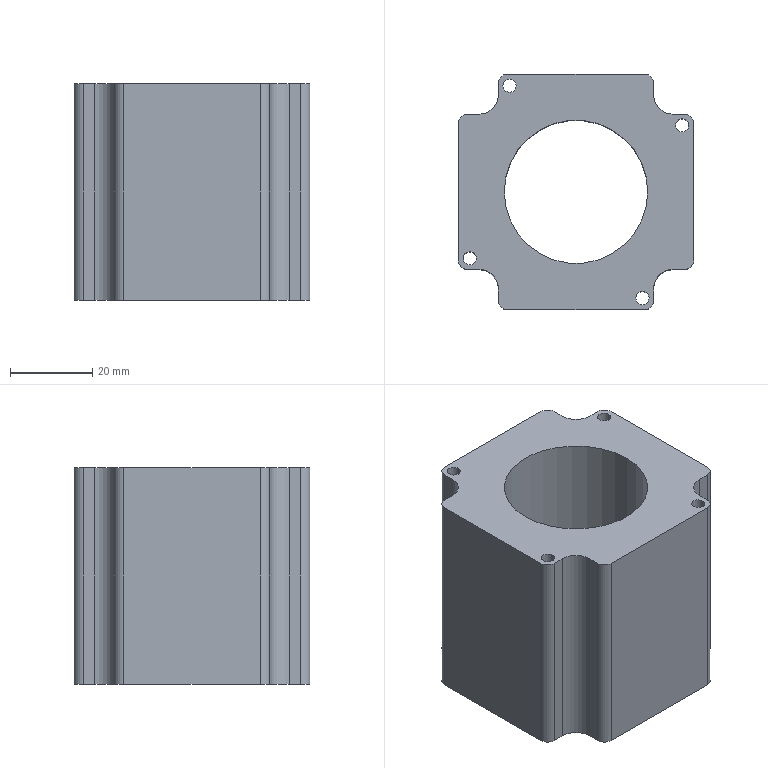Part | NX | features BREP 1 | 1 solid | 36 faces | box 57.15 x 57.15 x 52.6 mm | volume 100652 mm3 | cylinder 22 | plane 14 | commonest cylinder face diameters 3.2 x8 4.6 x8 9.5 x4 34.78 x2
STEP:
#1=CARTESIAN_POINT('',(17.39,0.,52.6));
#2=VERTEX_POINT('',#1);
#3=CARTESIAN_POINT('',(-17.39,0.,52.6));
#4=VERTEX_POINT('',#3);
#5=CARTESIAN_POINT('',(0.,0.,52.6));
#6=DIRECTION('',(0.,0.,-1.));
#7=DIRECTION('',(-1.,0.,0.));
#8=AXIS2_PLACEMENT_3D('',#5,#6,#7);
#9=CIRCLE('',#8,17.39);
#10=EDGE_CURVE('',#2,#4,#9,.T.);
#11=ORIENTED_EDGE('',*,*,#10,.F.);
#12=CARTESIAN_POINT('',(17.39,0.,0.));
#13=VERTEX_POINT('',#12);
#14=CARTESIAN_POINT('',(17.39,0.,52.6));
#15=DIRECTION('',(0.,0.,-1.));
#16=VECTOR('',#15,1000.);
#17=LINE('',#14,#16);
#18=EDGE_CURVE('',#13,#2,#17,.F.);
#19=ORIENTED_EDGE('',*,*,#18,.F.);
#20=CARTESIAN_POINT('',(-17.39,0.,0.));
#21=VERTEX_POINT('',#20);
#22=CARTESIAN_POINT('',(0.,0.,0.));
#23=DIRECTION('',(0.,0.,1.));
#24=DIRECTION('',(-1.,0.,0.));
#25=AXIS2_PLACEMENT_3D('',#22,#23,#24);
#26=CIRCLE('',#25,17.39);
#27=EDGE_CURVE('',#21,#13,#26,.T.);
#28=ORIENTED_EDGE('',*,*,#27,.F.);
#29=CARTESIAN_POINT('',(-17.39,0.,52.6));
#30=DIRECTION('',(0.,0.,-1.));
#31=VECTOR('',#30,1000.);
#32=LINE('',#29,#31);
#33=EDGE_CURVE('',#21,#4,#32,.F.);
#34=ORIENTED_EDGE('',*,*,#33,.T.);
#35=EDGE_LOOP('',(#11,#19,#28,#34));
#36=FACE_BOUND('',#35,.T.);
#37=CARTESIAN_POINT('',(0.,0.,52.6));
#38=DIRECTION('',(0.,0.,-1.));
#39=DIRECTION('',(1.,0.,0.));
#40=AXIS2_PLACEMENT_3D('',#37,#38,#39);
#41=CYLINDRICAL_SURFACE('',#40,17.39);
#42=ADVANCED_FACE('',(#36),#41,.F.);
#43=CARTESIAN_POINT('',(-14.51,25.75,0.));
#44=VERTEX_POINT('',#43);
#45=CARTESIAN_POINT('',(-17.71,25.75,0.));
#46=VERTEX_POINT('',#45);
#47=CARTESIAN_POINT('',(-16.11,25.75,0.));
#48=DIRECTION('',(0.,0.,-1.));
#49=DIRECTION('',(1.,0.,0.));
#50=AXIS2_PLACEMENT_3D('',#47,#48,#49);
#51=CIRCLE('',#50,1.6);
#52=EDGE_CURVE('',#44,#46,#51,.T.);
#53=ORIENTED_EDGE('',*,*,#52,.T.);
#54=CARTESIAN_POINT('',(-17.71,25.75,52.6));
#55=VERTEX_POINT('',#54);
#56=CARTESIAN_POINT('',(-17.71,25.75,0.));
#57=DIRECTION('',(0.,0.,1.));
#58=VECTOR('',#57,1000.);
#59=LINE('',#56,#58);
#60=EDGE_CURVE('',#46,#55,#59,.T.);
#61=ORIENTED_EDGE('',*,*,#60,.T.);
#62=CARTESIAN_POINT('',(-14.51,25.75,52.6));
#63=VERTEX_POINT('',#62);
#64=CARTESIAN_POINT('',(-16.11,25.75,52.6));
#65=DIRECTION('',(0.,0.,-1.));
#66=DIRECTION('',(1.,0.,0.));
#67=AXIS2_PLACEMENT_3D('',#64,#65,#66);
#68=CIRCLE('',#67,1.6);
#69=EDGE_CURVE('',#63,#55,#68,.T.);
#70=ORIENTED_EDGE('',*,*,#69,.F.);
#71=CARTESIAN_POINT('',(-14.51,25.75,0.));
#72=DIRECTION('',(0.,0.,1.));
#73=VECTOR('',#72,1000.);
#74=LINE('',#71,#73);
#75=EDGE_CURVE('',#44,#63,#74,.T.);
#76=ORIENTED_EDGE('',*,*,#75,.F.);
#77=EDGE_LOOP('',(#53,#61,#70,#76));
#78=FACE_BOUND('',#77,.T.);
#79=CARTESIAN_POINT('',(-16.11,25.75,0.));
#80=DIRECTION('',(0.,0.,1.));
#81=DIRECTION('',(-1.,0.,0.));
#82=AXIS2_PLACEMENT_3D('',#79,#80,#81);
#83=CYLINDRICAL_SURFACE('',#82,1.6);
#84=ADVANCED_FACE('',(#78),#83,.F.);
#85=CARTESIAN_POINT('',(27.35,16.11,0.));
#86=VERTEX_POINT('',#85);
#87=CARTESIAN_POINT('',(24.15,16.11,0.));
#88=VERTEX_POINT('',#87);
#89=CARTESIAN_POINT('',(25.75,16.11,0.));
#90=DIRECTION('',(0.,0.,-1.));
#91=DIRECTION('',(1.,0.,0.));
#92=AXIS2_PLACEMENT_3D('',#89,#90,#91);
#93=CIRCLE('',#92,1.6);
#94=EDGE_CURVE('',#86,#88,#93,.T.);
#95=ORIENTED_EDGE('',*,*,#94,.T.);
#96=CARTESIAN_POINT('',(24.15,16.11,52.6));
#97=VERTEX_POINT('',#96);
#98=CARTESIAN_POINT('',(24.15,16.11,0.));
#99=DIRECTION('',(0.,0.,1.));
#100=VECTOR('',#99,1000.);
#101=LINE('',#98,#100);
#102=EDGE_CURVE('',#88,#97,#101,.T.);
#103=ORIENTED_EDGE('',*,*,#102,.T.);
#104=CARTESIAN_POINT('',(27.35,16.11,52.6));
#105=VERTEX_POINT('',#104);
#106=CARTESIAN_POINT('',(25.75,16.11,52.6));
#107=DIRECTION('',(0.,0.,-1.));
#108=DIRECTION('',(1.,0.,0.));
#109=AXIS2_PLACEMENT_3D('',#106,#107,#108);
#110=CIRCLE('',#109,1.6);
#111=EDGE_CURVE('',#105,#97,#110,.T.);
#112=ORIENTED_EDGE('',*,*,#111,.F.);
#113=CARTESIAN_POINT('',(27.35,16.11,0.));
#114=DIRECTION('',(0.,0.,1.));
#115=VECTOR('',#114,1000.);
#116=LINE('',#113,#115);
#117=EDGE_CURVE('',#86,#105,#116,.T.);
#118=ORIENTED_EDGE('',*,*,#117,.F.);
#119=EDGE_LOOP('',(#95,#103,#112,#118));
#120=FACE_BOUND('',#119,.T.);
#121=CARTESIAN_POINT('',(25.75,16.11,0.));
#122=DIRECTION('',(0.,0.,1.));
#123=DIRECTION('',(-1.,0.,0.));
#124=AXIS2_PLACEMENT_3D('',#121,#122,#123);
#125=CYLINDRICAL_SURFACE('',#124,1.6);
#126=ADVANCED_FACE('',(#120),#125,.F.);
#127=CARTESIAN_POINT('',(17.71,-25.75,0.));
#128=VERTEX_POINT('',#127);
#129=CARTESIAN_POINT('',(14.51,-25.75,0.));
#130=VERTEX_POINT('',#129);
#131=CARTESIAN_POINT('',(16.11,-25.75,0.));
#132=DIRECTION('',(0.,0.,-1.));
#133=DIRECTION('',(1.,0.,0.));
#134=AXIS2_PLACEMENT_3D('',#131,#132,#133);
#135=CIRCLE('',#134,1.6);
#136=EDGE_CURVE('',#128,#130,#135,.T.);
#137=ORIENTED_EDGE('',*,*,#136,.T.);
#138=CARTESIAN_POINT('',(14.51,-25.75,52.6));
#139=VERTEX_POINT('',#138);
#140=CARTESIAN_POINT('',(14.51,-25.75,0.));
#141=DIRECTION('',(0.,0.,1.));
#142=VECTOR('',#141,1000.);
#143=LINE('',#140,#142);
#144=EDGE_CURVE('',#130,#139,#143,.T.);
#145=ORIENTED_EDGE('',*,*,#144,.T.);
#146=CARTESIAN_POINT('',(17.71,-25.75,52.6));
#147=VERTEX_POINT('',#146);
#148=CARTESIAN_POINT('',(16.11,-25.75,52.6));
#149=DIRECTION('',(0.,0.,-1.));
#150=DIRECTION('',(1.,0.,0.));
#151=AXIS2_PLACEMENT_3D('',#148,#149,#150);
#152=CIRCLE('',#151,1.6);
#153=EDGE_CURVE('',#147,#139,#152,.T.);
#154=ORIENTED_EDGE('',*,*,#153,.F.);
#155=CARTESIAN_POINT('',(17.71,-25.75,0.));
#156=DIRECTION('',(0.,0.,1.));
#157=VECTOR('',#156,1000.);
#158=LINE('',#155,#157);
#159=EDGE_CURVE('',#128,#147,#158,.T.);
#160=ORIENTED_EDGE('',*,*,#159,.F.);
#161=EDGE_LOOP('',(#137,#145,#154,#160));
#162=FACE_BOUND('',#161,.T.);
#163=CARTESIAN_POINT('',(16.11,-25.75,0.));
#164=DIRECTION('',(0.,0.,1.));
#165=DIRECTION('',(-1.,0.,0.));
#166=AXIS2_PLACEMENT_3D('',#163,#164,#165);
#167=CYLINDRICAL_SURFACE('',#166,1.6);
#168=ADVANCED_FACE('',(#162),#167,.F.);
#169=CARTESIAN_POINT('',(-24.15,-16.11,0.));
#170=VERTEX_POINT('',#169);
#171=CARTESIAN_POINT('',(-27.35,-16.11,0.));
#172=VERTEX_POINT('',#171);
#173=CARTESIAN_POINT('',(-25.75,-16.11,0.));
#174=DIRECTION('',(0.,0.,-1.));
#175=DIRECTION('',(1.,0.,0.));
#176=AXIS2_PLACEMENT_3D('',#173,#174,#175);
#177=CIRCLE('',#176,1.6);
#178=EDGE_CURVE('',#170,#172,#177,.T.);
#179=ORIENTED_EDGE('',*,*,#178,.T.);
#180=CARTESIAN_POINT('',(-27.35,-16.11,52.6));
#181=VERTEX_POINT('',#180);
#182=CARTESIAN_POINT('',(-27.35,-16.11,0.));
#183=DIRECTION('',(0.,0.,1.));
#184=VECTOR('',#183,1000.);
#185=LINE('',#182,#184);
#186=EDGE_CURVE('',#172,#181,#185,.T.);
#187=ORIENTED_EDGE('',*,*,#186,.T.);
#188=CARTESIAN_POINT('',(-24.15,-16.11,52.6));
#189=VERTEX_POINT('',#188);
#190=CARTESIAN_POINT('',(-25.75,-16.11,52.6));
#191=DIRECTION('',(0.,0.,-1.));
#192=DIRECTION('',(1.,0.,0.));
#193=AXIS2_PLACEMENT_3D('',#190,#191,#192);
#194=CIRCLE('',#193,1.6);
#195=EDGE_CURVE('',#189,#181,#194,.T.);
#196=ORIENTED_EDGE('',*,*,#195,.F.);
#197=CARTESIAN_POINT('',(-24.15,-16.11,0.));
#198=DIRECTION('',(0.,0.,1.));
#199=VECTOR('',#198,1000.);
#200=LINE('',#197,#199);
#201=EDGE_CURVE('',#170,#189,#200,.T.);
#202=ORIENTED_EDGE('',*,*,#201,.F.);
#203=EDGE_LOOP('',(#179,#187,#196,#202));
#204=FACE_BOUND('',#203,.T.);
#205=CARTESIAN_POINT('',(-25.75,-16.11,0.));
#206=DIRECTION('',(0.,0.,1.));
#207=DIRECTION('',(-1.,0.,0.));
#208=AXIS2_PLACEMENT_3D('',#205,#206,#207);
#209=CYLINDRICAL_SURFACE('',#208,1.6);
#210=ADVANCED_FACE('',(#204),#209,.F.);
#211=ORIENTED_EDGE('',*,*,#18,.T.);
#212=CARTESIAN_POINT('',(0.,0.,52.6));
#213=DIRECTION('',(0.,0.,-1.));
#214=DIRECTION('',(-1.,0.,0.));
#215=AXIS2_PLACEMENT_3D('',#212,#213,#214);
#216=CIRCLE('',#215,17.39);
#217=EDGE_CURVE('',#4,#2,#216,.T.);
#218=ORIENTED_EDGE('',*,*,#217,.F.);
#219=ORIENTED_EDGE('',*,*,#33,.F.);
#220=CARTESIAN_POINT('',(0.,0.,0.));
#221=DIRECTION('',(0.,0.,1.));
#222=DIRECTION('',(-1.,0.,0.));
#223=AXIS2_PLACEMENT_3D('',#220,#221,#222);
#224=CIRCLE('',#223,17.39);
#225=EDGE_CURVE('',#13,#21,#224,.T.);
#226=ORIENTED_EDGE('',*,*,#225,.F.);
#227=EDGE_LOOP('',(#211,#218,#219,#226));
#228=FACE_BOUND('',#227,.T.);
#229=CARTESIAN_POINT('',(0.,0.,52.6));
#230=DIRECTION('',(0.,0.,-1.));
#231=DIRECTION('',(1.,0.,0.));
#232=AXIS2_PLACEMENT_3D('',#229,#230,#231);
#233=CYLINDRICAL_SURFACE('',#232,17.39);
#234=ADVANCED_FACE('',(#228),#233,.F.);
#235=CARTESIAN_POINT('',(-18.82,-26.275,0.));
#236=VERTEX_POINT('',#235);
#237=CARTESIAN_POINT('',(-16.52,-28.575,0.));
#238=VERTEX_POINT('',#237);
#239=CARTESIAN_POINT('',(-16.52,-26.275,0.));
#240=DIRECTION('',(0.,0.,1.));
#241=DIRECTION('',(-1.,0.,0.));
#242=AXIS2_PLACEMENT_3D('',#239,#240,#241);
#243=CIRCLE('',#242,2.3);
#244=EDGE_CURVE('',#236,#238,#243,.T.);
#245=ORIENTED_EDGE('',*,*,#244,.F.);
#246=CARTESIAN_POINT('',(-18.82,-23.57,0.));
#247=VERTEX_POINT('',#246);
#248=CARTESIAN_POINT('',(-18.82,26.275,0.));
#249=DIRECTION('',(0.,-1.,0.));
#250=VECTOR('',#249,1000.);
#251=LINE('',#248,#250);
#252=EDGE_CURVE('',#247,#236,#251,.T.);
#253=ORIENTED_EDGE('',*,*,#252,.F.);
#254=CARTESIAN_POINT('',(-23.57,-18.82,0.));
#255=VERTEX_POINT('',#254);
#256=CARTESIAN_POINT('',(-23.57,-23.57,0.));
#257=DIRECTION('',(0.,0.,-1.));
#258=DIRECTION('',(-1.,0.,0.));
#259=AXIS2_PLACEMENT_3D('',#256,#257,#258);
#260=CIRCLE('',#259,4.75);
#261=EDGE_CURVE('',#255,#247,#260,.T.);
#262=ORIENTED_EDGE('',*,*,#261,.F.);
#263=CARTESIAN_POINT('',(-26.275,-18.82,0.));
#264=VERTEX_POINT('',#263);
#265=CARTESIAN_POINT('',(26.275,-18.82,0.));
#266=DIRECTION('',(1.,0.,0.));
#267=VECTOR('',#266,1000.);
#268=LINE('',#265,#267);
#269=EDGE_CURVE('',#264,#255,#268,.T.);
#270=ORIENTED_EDGE('',*,*,#269,.F.);
#271=CARTESIAN_POINT('',(-28.575,-16.52,0.));
#272=VERTEX_POINT('',#271);
#273=CARTESIAN_POINT('',(-26.275,-16.52,0.));
#274=DIRECTION('',(0.,0.,1.));
#275=DIRECTION('',(-1.,0.,0.));
#276=AXIS2_PLACEMENT_3D('',#273,#274,#275);
#277=CIRCLE('',#276,2.3);
#278=EDGE_CURVE('',#272,#264,#277,.T.);
#279=ORIENTED_EDGE('',*,*,#278,.F.);
#280=CARTESIAN_POINT('',(-28.575,16.52,0.));
#281=VERTEX_POINT('',#280);
#282=CARTESIAN_POINT('',(-28.575,26.275,0.));
#283=DIRECTION('',(0.,-1.,0.));
#284=VECTOR('',#283,1000.);
#285=LINE('',#282,#284);
#286=EDGE_CURVE('',#281,#272,#285,.T.);
#287=ORIENTED_EDGE('',*,*,#286,.F.);
#288=CARTESIAN_POINT('',(-26.275,18.82,0.));
#289=VERTEX_POINT('',#288);
#290=CARTESIAN_POINT('',(-26.275,16.52,0.));
#291=DIRECTION('',(0.,0.,1.));
#292=DIRECTION('',(-1.,0.,0.));
#293=AXIS2_PLACEMENT_3D('',#290,#291,#292);
#294=CIRCLE('',#293,2.3);
#295=EDGE_CURVE('',#289,#281,#294,.T.);
#296=ORIENTED_EDGE('',*,*,#295,.F.);
#297=CARTESIAN_POINT('',(-23.57,18.82,0.));
#298=VERTEX_POINT('',#297);
#299=CARTESIAN_POINT('',(26.275,18.82,0.));
#300=DIRECTION('',(-1.,0.,0.));
#301=VECTOR('',#300,1000.);
#302=LINE('',#299,#301);
#303=EDGE_CURVE('',#298,#289,#302,.T.);
#304=ORIENTED_EDGE('',*,*,#303,.F.);
#305=CARTESIAN_POINT('',(-18.82,23.57,0.));
#306=VERTEX_POINT('',#305);
#307=CARTESIAN_POINT('',(-23.57,23.57,0.));
#308=DIRECTION('',(0.,0.,-1.));
#309=DIRECTION('',(-1.,0.,0.));
#310=AXIS2_PLACEMENT_3D('',#307,#308,#309);
#311=CIRCLE('',#310,4.75);
#312=EDGE_CURVE('',#306,#298,#311,.T.);
#313=ORIENTED_EDGE('',*,*,#312,.F.);
#314=CARTESIAN_POINT('',(-18.82,26.275,0.));
#315=VERTEX_POINT('',#314);
#316=CARTESIAN_POINT('',(-18.82,26.275,0.));
#317=DIRECTION('',(0.,-1.,0.));
#318=VECTOR('',#317,1000.);
#319=LINE('',#316,#318);
#320=EDGE_CURVE('',#315,#306,#319,.T.);
#321=ORIENTED_EDGE('',*,*,#320,.F.);
#322=CARTESIAN_POINT('',(-16.52,28.575,0.));
#323=VERTEX_POINT('',#322);
#324=CARTESIAN_POINT('',(-16.52,26.275,0.));
#325=DIRECTION('',(0.,0.,1.));
#326=DIRECTION('',(-1.,0.,0.));
#327=AXIS2_PLACEMENT_3D('',#324,#325,#326);
#328=CIRCLE('',#327,2.3);
#329=EDGE_CURVE('',#323,#315,#328,.T.);
#330=ORIENTED_EDGE('',*,*,#329,.F.);
#331=CARTESIAN_POINT('',(16.52,28.575,0.));
#332=VERTEX_POINT('',#331);
#333=CARTESIAN_POINT('',(26.275,28.575,0.));
#334=DIRECTION('',(-1.,0.,0.));
#335=VECTOR('',#334,1000.);
#336=LINE('',#333,#335);
#337=EDGE_CURVE('',#332,#323,#336,.T.);
#338=ORIENTED_EDGE('',*,*,#337,.F.);
#339=CARTESIAN_POINT('',(18.82,26.275,0.));
#340=VERTEX_POINT('',#339);
#341=CARTESIAN_POINT('',(16.52,26.275,0.));
#342=DIRECTION('',(0.,0.,1.));
#343=DIRECTION('',(-1.,0.,0.));
#344=AXIS2_PLACEMENT_3D('',#341,#342,#343);
#345=CIRCLE('',#344,2.3);
#346=EDGE_CURVE('',#340,#332,#345,.T.);
#347=ORIENTED_EDGE('',*,*,#346,.F.);
#348=CARTESIAN_POINT('',(18.82,23.57,0.));
#349=VERTEX_POINT('',#348);
#350=CARTESIAN_POINT('',(18.82,26.275,0.));
#351=DIRECTION('',(0.,1.,0.));
#352=VECTOR('',#351,1000.);
#353=LINE('',#350,#352);
#354=EDGE_CURVE('',#349,#340,#353,.T.);
#355=ORIENTED_EDGE('',*,*,#354,.F.);
#356=CARTESIAN_POINT('',(23.57,18.82,0.));
#357=VERTEX_POINT('',#356);
#358=CARTESIAN_POINT('',(23.57,23.57,0.));
#359=DIRECTION('',(0.,0.,-1.));
#360=DIRECTION('',(-1.,0.,0.));
#361=AXIS2_PLACEMENT_3D('',#358,#359,#360);
#362=CIRCLE('',#361,4.75);
#363=EDGE_CURVE('',#357,#349,#362,.T.);
#364=ORIENTED_EDGE('',*,*,#363,.F.);
#365=CARTESIAN_POINT('',(26.275,18.82,0.));
#366=VERTEX_POINT('',#365);
#367=CARTESIAN_POINT('',(26.275,18.82,0.));
#368=DIRECTION('',(-1.,0.,0.));
#369=VECTOR('',#368,1000.);
#370=LINE('',#367,#369);
#371=EDGE_CURVE('',#366,#357,#370,.T.);
#372=ORIENTED_EDGE('',*,*,#371,.F.);
#373=CARTESIAN_POINT('',(28.575,16.52,0.));
#374=VERTEX_POINT('',#373);
#375=CARTESIAN_POINT('',(26.275,16.52,0.));
#376=DIRECTION('',(0.,0.,1.));
#377=DIRECTION('',(-1.,0.,0.));
#378=AXIS2_PLACEMENT_3D('',#375,#376,#377);
#379=CIRCLE('',#378,2.3);
#380=EDGE_CURVE('',#374,#366,#379,.T.);
#381=ORIENTED_EDGE('',*,*,#380,.F.);
#382=CARTESIAN_POINT('',(28.575,-16.52,0.));
#383=VERTEX_POINT('',#382);
#384=CARTESIAN_POINT('',(28.575,26.275,0.));
#385=DIRECTION('',(0.,1.,0.));
#386=VECTOR('',#385,1000.);
#387=LINE('',#384,#386);
#388=EDGE_CURVE('',#383,#374,#387,.T.);
#389=ORIENTED_EDGE('',*,*,#388,.F.);
#390=CARTESIAN_POINT('',(26.275,-18.82,0.));
#391=VERTEX_POINT('',#390);
#392=CARTESIAN_POINT('',(26.275,-16.52,0.));
#393=DIRECTION('',(0.,0.,1.));
#394=DIRECTION('',(-1.,0.,0.));
#395=AXIS2_PLACEMENT_3D('',#392,#393,#394);
#396=CIRCLE('',#395,2.3);
#397=EDGE_CURVE('',#391,#383,#396,.T.);
#398=ORIENTED_EDGE('',*,*,#397,.F.);
#399=CARTESIAN_POINT('',(23.57,-18.82,0.));
#400=VERTEX_POINT('',#399);
#401=CARTESIAN_POINT('',(26.275,-18.82,0.));
#402=DIRECTION('',(1.,0.,0.));
#403=VECTOR('',#402,1000.);
#404=LINE('',#401,#403);
#405=EDGE_CURVE('',#400,#391,#404,.T.);
#406=ORIENTED_EDGE('',*,*,#405,.F.);
#407=CARTESIAN_POINT('',(18.82,-23.57,0.));
#408=VERTEX_POINT('',#407);
#409=CARTESIAN_POINT('',(23.57,-23.57,0.));
#410=DIRECTION('',(0.,0.,-1.));
#411=DIRECTION('',(-1.,0.,0.));
#412=AXIS2_PLACEMENT_3D('',#409,#410,#411);
#413=CIRCLE('',#412,4.75);
#414=EDGE_CURVE('',#408,#400,#413,.T.);
#415=ORIENTED_EDGE('',*,*,#414,.F.);
#416=CARTESIAN_POINT('',(18.82,-26.275,0.));
#417=VERTEX_POINT('',#416);
#418=CARTESIAN_POINT('',(18.82,26.275,0.));
#419=DIRECTION('',(0.,1.,0.));
#420=VECTOR('',#419,1000.);
#421=LINE('',#418,#420);
#422=EDGE_CURVE('',#417,#408,#421,.T.);
#423=ORIENTED_EDGE('',*,*,#422,.F.);
#424=CARTESIAN_POINT('',(16.52,-28.575,0.));
#425=VERTEX_POINT('',#424);
#426=CARTESIAN_POINT('',(16.52,-26.275,0.));
#427=DIRECTION('',(0.,0.,1.));
#428=DIRECTION('',(-1.,0.,0.));
#429=AXIS2_PLACEMENT_3D('',#426,#427,#428);
#430=CIRCLE('',#429,2.3);
#431=EDGE_CURVE('',#425,#417,#430,.T.);
#432=ORIENTED_EDGE('',*,*,#431,.F.);
#433=CARTESIAN_POINT('',(26.275,-28.575,0.));
#434=DIRECTION('',(1.,0.,0.));
#435=VECTOR('',#434,1000.);
#436=LINE('',#433,#435);
#437=EDGE_CURVE('',#238,#425,#436,.T.);
#438=ORIENTED_EDGE('',*,*,#437,.F.);
#439=EDGE_LOOP('',(#245,#253,#262,#270,#279,#287,#296,#304,#313,#321,#330,#338,#347,#355,#364,#372,#381,#389,#398,#406,#415,#423,#432,#438));
#440=FACE_BOUND('',#439,.T.);
#441=ORIENTED_EDGE('',*,*,#52,.F.);
#442=CARTESIAN_POINT('',(-16.11,25.75,0.));
#443=DIRECTION('',(0.,0.,-1.));
#444=DIRECTION('',(1.,0.,0.));
#445=AXIS2_PLACEMENT_3D('',#442,#443,#444);
#446=CIRCLE('',#445,1.6);
#447=EDGE_CURVE('',#46,#44,#446,.T.);
#448=ORIENTED_EDGE('',*,*,#447,.F.);
#449=EDGE_LOOP('',(#441,#448));
#450=FACE_BOUND('',#449,.T.);
#451=ORIENTED_EDGE('',*,*,#94,.F.);
#452=CARTESIAN_POINT('',(25.75,16.11,0.));
#453=DIRECTION('',(0.,0.,-1.));
#454=DIRECTION('',(1.,0.,0.));
#455=AXIS2_PLACEMENT_3D('',#452,#453,#454);
#456=CIRCLE('',#455,1.6);
#457=EDGE_CURVE('',#88,#86,#456,.T.);
#458=ORIENTED_EDGE('',*,*,#457,.F.);
#459=EDGE_LOOP('',(#451,#458));
#460=FACE_BOUND('',#459,.T.);
#461=ORIENTED_EDGE('',*,*,#136,.F.);
#462=CARTESIAN_POINT('',(16.11,-25.75,0.));
#463=DIRECTION('',(0.,0.,-1.));
#464=DIRECTION('',(1.,0.,0.));
#465=AXIS2_PLACEMENT_3D('',#462,#463,#464);
#466=CIRCLE('',#465,1.6);
#467=EDGE_CURVE('',#130,#128,#466,.T.);
#468=ORIENTED_EDGE('',*,*,#467,.F.);
#469=EDGE_LOOP('',(#461,#468));
#470=FACE_BOUND('',#469,.T.);
#471=ORIENTED_EDGE('',*,*,#178,.F.);
#472=CARTESIAN_POINT('',(-25.75,-16.11,0.));
#473=DIRECTION('',(0.,0.,-1.));
#474=DIRECTION('',(1.,0.,0.));
#475=AXIS2_PLACEMENT_3D('',#472,#473,#474);
#476=CIRCLE('',#475,1.6);
#477=EDGE_CURVE('',#172,#170,#476,.T.);
#478=ORIENTED_EDGE('',*,*,#477,.F.);
#479=EDGE_LOOP('',(#471,#478));
#480=FACE_BOUND('',#479,.T.);
#481=ORIENTED_EDGE('',*,*,#27,.T.);
#482=ORIENTED_EDGE('',*,*,#225,.T.);
#483=EDGE_LOOP('',(#481,#482));
#484=FACE_BOUND('',#483,.T.);
#485=CARTESIAN_POINT('',(26.275,26.275,0.));
#486=DIRECTION('',(0.,0.,1.));
#487=DIRECTION('',(-1.,0.,0.));
#488=AXIS2_PLACEMENT_3D('',#485,#486,#487);
#489=PLANE('',#488);
#490=ADVANCED_FACE('',(#440,#450,#460,#470,#480,#484),#489,.F.);
#491=CARTESIAN_POINT('',(-23.57,-18.82,52.6));
#492=VERTEX_POINT('',#491);
#493=CARTESIAN_POINT('',(-18.82,-23.57,52.6));
#494=VERTEX_POINT('',#493);
#495=CARTESIAN_POINT('',(-23.57,-23.57,52.6));
#496=DIRECTION('',(0.,0.,-1.));
#497=DIRECTION('',(-1.,0.,0.));
#498=AXIS2_PLACEMENT_3D('',#495,#496,#497);
#499=CIRCLE('',#498,4.75);
#500=EDGE_CURVE('',#492,#494,#499,.T.);
#501=ORIENTED_EDGE('',*,*,#500,.T.);
#502=CARTESIAN_POINT('',(-18.82,-26.275,52.6));
#503=VERTEX_POINT('',#502);
#504=CARTESIAN_POINT('',(-18.82,26.275,52.6));
#505=DIRECTION('',(0.,-1.,0.));
#506=VECTOR('',#505,1000.);
#507=LINE('',#504,#506);
#508=EDGE_CURVE('',#494,#503,#507,.T.);
#509=ORIENTED_EDGE('',*,*,#508,.T.);
#510=CARTESIAN_POINT('',(-16.52,-28.575,52.6));
#511=VERTEX_POINT('',#510);
#512=CARTESIAN_POINT('',(-16.52,-26.275,52.6));
#513=DIRECTION('',(0.,0.,1.));
#514=DIRECTION('',(-1.,0.,0.));
#515=AXIS2_PLACEMENT_3D('',#512,#513,#514);
#516=CIRCLE('',#515,2.3);
#517=EDGE_CURVE('',#503,#511,#516,.T.);
#518=ORIENTED_EDGE('',*,*,#517,.T.);
#519=CARTESIAN_POINT('',(16.52,-28.575,52.6));
#520=VERTEX_POINT('',#519);
#521=CARTESIAN_POINT('',(26.275,-28.575,52.6));
#522=DIRECTION('',(1.,0.,0.));
#523=VECTOR('',#522,1000.);
#524=LINE('',#521,#523);
#525=EDGE_CURVE('',#511,#520,#524,.T.);
#526=ORIENTED_EDGE('',*,*,#525,.T.);
#527=CARTESIAN_POINT('',(18.82,-26.275,52.6));
#528=VERTEX_POINT('',#527);
#529=CARTESIAN_POINT('',(16.52,-26.275,52.6));
#530=DIRECTION('',(0.,0.,1.));
#531=DIRECTION('',(-1.,0.,0.));
#532=AXIS2_PLACEMENT_3D('',#529,#530,#531);
#533=CIRCLE('',#532,2.3);
#534=EDGE_CURVE('',#520,#528,#533,.T.);
#535=ORIENTED_EDGE('',*,*,#534,.T.);
#536=CARTESIAN_POINT('',(18.82,-23.57,52.6));
#537=VERTEX_POINT('',#536);
#538=CARTESIAN_POINT('',(18.82,26.275,52.6));
#539=DIRECTION('',(0.,1.,0.));
#540=VECTOR('',#539,1000.);
#541=LINE('',#538,#540);
#542=EDGE_CURVE('',#528,#537,#541,.T.);
#543=ORIENTED_EDGE('',*,*,#542,.T.);
#544=CARTESIAN_POINT('',(23.57,-18.82,52.6));
#545=VERTEX_POINT('',#544);
#546=CARTESIAN_POINT('',(23.57,-23.57,52.6));
#547=DIRECTION('',(0.,0.,-1.));
#548=DIRECTION('',(-1.,0.,0.));
#549=AXIS2_PLACEMENT_3D('',#546,#547,#548);
#550=CIRCLE('',#549,4.75);
#551=EDGE_CURVE('',#537,#545,#550,.T.);
#552=ORIENTED_EDGE('',*,*,#551,.T.);
#553=CARTESIAN_POINT('',(26.275,-18.82,52.6));
#554=VERTEX_POINT('',#553);
#555=CARTESIAN_POINT('',(26.275,-18.82,52.6));
#556=DIRECTION('',(1.,0.,0.));
#557=VECTOR('',#556,1000.);
#558=LINE('',#555,#557);
#559=EDGE_CURVE('',#545,#554,#558,.T.);
#560=ORIENTED_EDGE('',*,*,#559,.T.);
#561=CARTESIAN_POINT('',(28.575,-16.52,52.6));
#562=VERTEX_POINT('',#561);
#563=CARTESIAN_POINT('',(26.275,-16.52,52.6));
#564=DIRECTION('',(0.,0.,1.));
#565=DIRECTION('',(-1.,0.,0.));
#566=AXIS2_PLACEMENT_3D('',#563,#564,#565);
#567=CIRCLE('',#566,2.3);
#568=EDGE_CURVE('',#554,#562,#567,.T.);
#569=ORIENTED_EDGE('',*,*,#568,.T.);
#570=CARTESIAN_POINT('',(28.575,16.52,52.6));
#571=VERTEX_POINT('',#570);
#572=CARTESIAN_POINT('',(28.575,26.275,52.6));
#573=DIRECTION('',(0.,1.,0.));
#574=VECTOR('',#573,1000.);
#575=LINE('',#572,#574);
#576=EDGE_CURVE('',#562,#571,#575,.T.);
#577=ORIENTED_EDGE('',*,*,#576,.T.);
#578=CARTESIAN_POINT('',(26.275,18.82,52.6));
#579=VERTEX_POINT('',#578);
#580=CARTESIAN_POINT('',(26.275,16.52,52.6));
#581=DIRECTION('',(0.,0.,1.));
#582=DIRECTION('',(-1.,0.,0.));
#583=AXIS2_PLACEMENT_3D('',#580,#581,#582);
#584=CIRCLE('',#583,2.3);
#585=EDGE_CURVE('',#571,#579,#584,.T.);
#586=ORIENTED_EDGE('',*,*,#585,.T.);
#587=CARTESIAN_POINT('',(23.57,18.82,52.6));
#588=VERTEX_POINT('',#587);
#589=CARTESIAN_POINT('',(26.275,18.82,52.6));
#590=DIRECTION('',(-1.,0.,0.));
#591=VECTOR('',#590,1000.);
#592=LINE('',#589,#591);
#593=EDGE_CURVE('',#579,#588,#592,.T.);
#594=ORIENTED_EDGE('',*,*,#593,.T.);
#595=CARTESIAN_POINT('',(18.82,23.57,52.6));
#596=VERTEX_POINT('',#595);
#597=CARTESIAN_POINT('',(23.57,23.57,52.6));
#598=DIRECTION('',(0.,0.,-1.));
#599=DIRECTION('',(-1.,0.,0.));
#600=AXIS2_PLACEMENT_3D('',#597,#598,#599);
#601=CIRCLE('',#600,4.75);
#602=EDGE_CURVE('',#588,#596,#601,.T.);
#603=ORIENTED_EDGE('',*,*,#602,.T.);
#604=CARTESIAN_POINT('',(18.82,26.275,52.6));
#605=VERTEX_POINT('',#604);
#606=CARTESIAN_POINT('',(18.82,26.275,52.6));
#607=DIRECTION('',(0.,1.,0.));
#608=VECTOR('',#607,1000.);
#609=LINE('',#606,#608);
#610=EDGE_CURVE('',#596,#605,#609,.T.);
#611=ORIENTED_EDGE('',*,*,#610,.T.);
#612=CARTESIAN_POINT('',(16.52,28.575,52.6));
#613=VERTEX_POINT('',#612);
#614=CARTESIAN_POINT('',(16.52,26.275,52.6));
#615=DIRECTION('',(0.,0.,1.));
#616=DIRECTION('',(-1.,0.,0.));
#617=AXIS2_PLACEMENT_3D('',#614,#615,#616);
#618=CIRCLE('',#617,2.3);
#619=EDGE_CURVE('',#605,#613,#618,.T.);
#620=ORIENTED_EDGE('',*,*,#619,.T.);
#621=CARTESIAN_POINT('',(-16.52,28.575,52.6));
#622=VERTEX_POINT('',#621);
#623=CARTESIAN_POINT('',(26.275,28.575,52.6));
#624=DIRECTION('',(-1.,0.,0.));
#625=VECTOR('',#624,1000.);
#626=LINE('',#623,#625);
#627=EDGE_CURVE('',#613,#622,#626,.T.);
#628=ORIENTED_EDGE('',*,*,#627,.T.);
#629=CARTESIAN_POINT('',(-18.82,26.275,52.6));
#630=VERTEX_POINT('',#629);
#631=CARTESIAN_POINT('',(-16.52,26.275,52.6));
#632=DIRECTION('',(0.,0.,1.));
#633=DIRECTION('',(-1.,0.,0.));
#634=AXIS2_PLACEMENT_3D('',#631,#632,#633);
#635=CIRCLE('',#634,2.3);
#636=EDGE_CURVE('',#622,#630,#635,.T.);
#637=ORIENTED_EDGE('',*,*,#636,.T.);
#638=CARTESIAN_POINT('',(-18.82,23.57,52.6));
#639=VERTEX_POINT('',#638);
#640=CARTESIAN_POINT('',(-18.82,26.275,52.6));
#641=DIRECTION('',(0.,-1.,0.));
#642=VECTOR('',#641,1000.);
#643=LINE('',#640,#642);
#644=EDGE_CURVE('',#630,#639,#643,.T.);
#645=ORIENTED_EDGE('',*,*,#644,.T.);
#646=CARTESIAN_POINT('',(-23.57,18.82,52.6));
#647=VERTEX_POINT('',#646);
#648=CARTESIAN_POINT('',(-23.57,23.57,52.6));
#649=DIRECTION('',(0.,0.,-1.));
#650=DIRECTION('',(-1.,0.,0.));
#651=AXIS2_PLACEMENT_3D('',#648,#649,#650);
#652=CIRCLE('',#651,4.75);
#653=EDGE_CURVE('',#639,#647,#652,.T.);
#654=ORIENTED_EDGE('',*,*,#653,.T.);
#655=CARTESIAN_POINT('',(-26.275,18.82,52.6));
#656=VERTEX_POINT('',#655);
#657=CARTESIAN_POINT('',(26.275,18.82,52.6));
#658=DIRECTION('',(-1.,0.,0.));
#659=VECTOR('',#658,1000.);
#660=LINE('',#657,#659);
#661=EDGE_CURVE('',#647,#656,#660,.T.);
#662=ORIENTED_EDGE('',*,*,#661,.T.);
#663=CARTESIAN_POINT('',(-28.575,16.52,52.6));
#664=VERTEX_POINT('',#663);
#665=CARTESIAN_POINT('',(-26.275,16.52,52.6));
#666=DIRECTION('',(0.,0.,1.));
#667=DIRECTION('',(-1.,0.,0.));
#668=AXIS2_PLACEMENT_3D('',#665,#666,#667);
#669=CIRCLE('',#668,2.3);
#670=EDGE_CURVE('',#656,#664,#669,.T.);
#671=ORIENTED_EDGE('',*,*,#670,.T.);
#672=CARTESIAN_POINT('',(-28.575,-16.52,52.6));
#673=VERTEX_POINT('',#672);
#674=CARTESIAN_POINT('',(-28.575,26.275,52.6));
#675=DIRECTION('',(0.,-1.,0.));
#676=VECTOR('',#675,1000.);
#677=LINE('',#674,#676);
#678=EDGE_CURVE('',#664,#673,#677,.T.);
#679=ORIENTED_EDGE('',*,*,#678,.T.);
#680=CARTESIAN_POINT('',(-26.275,-18.82,52.6));
#681=VERTEX_POINT('',#680);
#682=CARTESIAN_POINT('',(-26.275,-16.52,52.6));
#683=DIRECTION('',(0.,0.,1.));
#684=DIRECTION('',(-1.,0.,0.));
#685=AXIS2_PLACEMENT_3D('',#682,#683,#684);
#686=CIRCLE('',#685,2.3);
#687=EDGE_CURVE('',#673,#681,#686,.T.);
#688=ORIENTED_EDGE('',*,*,#687,.T.);
#689=CARTESIAN_POINT('',(26.275,-18.82,52.6));
#690=DIRECTION('',(1.,0.,0.));
#691=VECTOR('',#690,1000.);
#692=LINE('',#689,#691);
#693=EDGE_CURVE('',#681,#492,#692,.T.);
#694=ORIENTED_EDGE('',*,*,#693,.T.);
#695=EDGE_LOOP('',(#501,#509,#518,#526,#535,#543,#552,#560,#569,#577,#586,#594,#603,#611,#620,#628,#637,#645,#654,#662,#671,#679,#688,#694));
#696=FACE_BOUND('',#695,.T.);
#697=ORIENTED_EDGE('',*,*,#69,.T.);
#698=CARTESIAN_POINT('',(-16.11,25.75,52.6));
#699=DIRECTION('',(0.,0.,-1.));
#700=DIRECTION('',(1.,0.,0.));
#701=AXIS2_PLACEMENT_3D('',#698,#699,#700);
#702=CIRCLE('',#701,1.6);
#703=EDGE_CURVE('',#55,#63,#702,.T.);
#704=ORIENTED_EDGE('',*,*,#703,.T.);
#705=EDGE_LOOP('',(#697,#704));
#706=FACE_BOUND('',#705,.T.);
#707=ORIENTED_EDGE('',*,*,#111,.T.);
#708=CARTESIAN_POINT('',(25.75,16.11,52.6));
#709=DIRECTION('',(0.,0.,-1.));
#710=DIRECTION('',(1.,0.,0.));
#711=AXIS2_PLACEMENT_3D('',#708,#709,#710);
#712=CIRCLE('',#711,1.6);
#713=EDGE_CURVE('',#97,#105,#712,.T.);
#714=ORIENTED_EDGE('',*,*,#713,.T.);
#715=EDGE_LOOP('',(#707,#714));
#716=FACE_BOUND('',#715,.T.);
#717=ORIENTED_EDGE('',*,*,#153,.T.);
#718=CARTESIAN_POINT('',(16.11,-25.75,52.6));
#719=DIRECTION('',(0.,0.,-1.));
#720=DIRECTION('',(1.,0.,0.));
#721=AXIS2_PLACEMENT_3D('',#718,#719,#720);
#722=CIRCLE('',#721,1.6);
#723=EDGE_CURVE('',#139,#147,#722,.T.);
#724=ORIENTED_EDGE('',*,*,#723,.T.);
#725=EDGE_LOOP('',(#717,#724));
#726=FACE_BOUND('',#725,.T.);
#727=ORIENTED_EDGE('',*,*,#195,.T.);
#728=CARTESIAN_POINT('',(-25.75,-16.11,52.6));
#729=DIRECTION('',(0.,0.,-1.));
#730=DIRECTION('',(1.,0.,0.));
#731=AXIS2_PLACEMENT_3D('',#728,#729,#730);
#732=CIRCLE('',#731,1.6);
#733=EDGE_CURVE('',#181,#189,#732,.T.);
#734=ORIENTED_EDGE('',*,*,#733,.T.);
#735=EDGE_LOOP('',(#727,#734));
#736=FACE_BOUND('',#735,.T.);
#737=ORIENTED_EDGE('',*,*,#217,.T.);
#738=ORIENTED_EDGE('',*,*,#10,.T.);
#739=EDGE_LOOP('',(#737,#738));
#740=FACE_BOUND('',#739,.T.);
#741=CARTESIAN_POINT('',(26.275,26.275,52.6));
#742=DIRECTION('',(0.,0.,1.));
#743=DIRECTION('',(-1.,0.,0.));
#744=AXIS2_PLACEMENT_3D('',#741,#742,#743);
#745=PLANE('',#744);
#746=ADVANCED_FACE('',(#696,#706,#716,#726,#736,#740),#745,.T.);
#747=ORIENTED_EDGE('',*,*,#437,.T.);
#748=CARTESIAN_POINT('',(16.52,-28.575,52.6));
#749=DIRECTION('',(0.,0.,-1.));
#750=VECTOR('',#749,1000.);
#751=LINE('',#748,#750);
#752=EDGE_CURVE('',#520,#425,#751,.T.);
#753=ORIENTED_EDGE('',*,*,#752,.F.);
#754=ORIENTED_EDGE('',*,*,#525,.F.);
#755=CARTESIAN_POINT('',(-16.52,-28.575,52.6));
#756=DIRECTION('',(0.,0.,1.));
#757=VECTOR('',#756,1000.);
#758=LINE('',#755,#757);
#759=EDGE_CURVE('',#238,#511,#758,.T.);
#760=ORIENTED_EDGE('',*,*,#759,.F.);
#761=EDGE_LOOP('',(#747,#753,#754,#760));
#762=FACE_BOUND('',#761,.T.);
#763=CARTESIAN_POINT('',(-26.275,-28.575,52.6));
#764=DIRECTION('',(0.,1.,0.));
#765=DIRECTION('',(0.,0.,-1.));
#766=AXIS2_PLACEMENT_3D('',#763,#764,#765);
#767=PLANE('',#766);
#768=ADVANCED_FACE('',(#762),#767,.F.);
#769=ORIENTED_EDGE('',*,*,#517,.F.);
#770=CARTESIAN_POINT('',(-18.82,-26.275,52.6));
#771=DIRECTION('',(0.,0.,-1.));
#772=VECTOR('',#771,1000.);
#773=LINE('',#770,#772);
#774=EDGE_CURVE('',#503,#236,#773,.T.);
#775=ORIENTED_EDGE('',*,*,#774,.T.);
#776=ORIENTED_EDGE('',*,*,#244,.T.);
#777=ORIENTED_EDGE('',*,*,#759,.T.);
#778=EDGE_LOOP('',(#769,#775,#776,#777));
#779=FACE_BOUND('',#778,.T.);
#780=CARTESIAN_POINT('',(-16.52,-26.275,52.6));
#781=DIRECTION('',(0.,0.,-1.));
#782=DIRECTION('',(1.,0.,0.));
#783=AXIS2_PLACEMENT_3D('',#780,#781,#782);
#784=CYLINDRICAL_SURFACE('',#783,2.3);
#785=ADVANCED_FACE('',(#779),#784,.T.);
#786=ORIENTED_EDGE('',*,*,#774,.F.);
#787=ORIENTED_EDGE('',*,*,#508,.F.);
#788=CARTESIAN_POINT('',(-18.82,-23.57,52.6));
#789=DIRECTION('',(0.,0.,1.));
#790=VECTOR('',#789,1000.);
#791=LINE('',#788,#790);
#792=EDGE_CURVE('',#247,#494,#791,.T.);
#793=ORIENTED_EDGE('',*,*,#792,.F.);
#794=ORIENTED_EDGE('',*,*,#252,.T.);
#795=EDGE_LOOP('',(#786,#787,#793,#794));
#796=FACE_BOUND('',#795,.T.);
#797=CARTESIAN_POINT('',(-18.82,-26.275,52.6));
#798=DIRECTION('',(1.,0.,0.));
#799=DIRECTION('',(0.,-1.,0.));
#800=AXIS2_PLACEMENT_3D('',#797,#798,#799);
#801=PLANE('',#800);
#802=ADVANCED_FACE('',(#796),#801,.F.);
#803=ORIENTED_EDGE('',*,*,#792,.T.);
#804=ORIENTED_EDGE('',*,*,#500,.F.);
#805=CARTESIAN_POINT('',(-23.57,-18.82,52.6));
#806=DIRECTION('',(0.,0.,1.));
#807=VECTOR('',#806,1000.);
#808=LINE('',#805,#807);
#809=EDGE_CURVE('',#255,#492,#808,.T.);
#810=ORIENTED_EDGE('',*,*,#809,.F.);
#811=ORIENTED_EDGE('',*,*,#261,.T.);
#812=EDGE_LOOP('',(#803,#804,#810,#811));
#813=FACE_BOUND('',#812,.T.);
#814=CARTESIAN_POINT('',(-23.57,-23.57,52.6));
#815=DIRECTION('',(0.,0.,-1.));
#816=DIRECTION('',(1.,0.,0.));
#817=AXIS2_PLACEMENT_3D('',#814,#815,#816);
#818=CYLINDRICAL_SURFACE('',#817,4.75);
#819=ADVANCED_FACE('',(#813),#818,.F.);
#820=ORIENTED_EDGE('',*,*,#809,.T.);
#821=ORIENTED_EDGE('',*,*,#693,.F.);
#822=CARTESIAN_POINT('',(-26.275,-18.82,52.6));
#823=DIRECTION('',(0.,0.,1.));
#824=VECTOR('',#823,1000.);
#825=LINE('',#822,#824);
#826=EDGE_CURVE('',#264,#681,#825,.T.);
#827=ORIENTED_EDGE('',*,*,#826,.F.);
#828=ORIENTED_EDGE('',*,*,#269,.T.);
#829=EDGE_LOOP('',(#820,#821,#827,#828));
#830=FACE_BOUND('',#829,.T.);
#831=CARTESIAN_POINT('',(-23.57,-18.82,52.6));
#832=DIRECTION('',(0.,1.,0.));
#833=DIRECTION('',(0.,0.,-1.));
#834=AXIS2_PLACEMENT_3D('',#831,#832,#833);
#835=PLANE('',#834);
#836=ADVANCED_FACE('',(#830),#835,.F.);
#837=ORIENTED_EDGE('',*,*,#687,.F.);
#838=CARTESIAN_POINT('',(-28.575,-16.52,52.6));
#839=DIRECTION('',(0.,0.,-1.));
#840=VECTOR('',#839,1000.);
#841=LINE('',#838,#840);
#842=EDGE_CURVE('',#673,#272,#841,.T.);
#843=ORIENTED_EDGE('',*,*,#842,.T.);
#844=ORIENTED_EDGE('',*,*,#278,.T.);
#845=ORIENTED_EDGE('',*,*,#826,.T.);
#846=EDGE_LOOP('',(#837,#843,#844,#845));
#847=FACE_BOUND('',#846,.T.);
#848=CARTESIAN_POINT('',(-26.275,-16.52,52.6));
#849=DIRECTION('',(0.,0.,-1.));
#850=DIRECTION('',(1.,0.,0.));
#851=AXIS2_PLACEMENT_3D('',#848,#849,#850);
#852=CYLINDRICAL_SURFACE('',#851,2.3);
#853=ADVANCED_FACE('',(#847),#852,.T.);
#854=ORIENTED_EDGE('',*,*,#842,.F.);
#855=ORIENTED_EDGE('',*,*,#678,.F.);
#856=CARTESIAN_POINT('',(-28.575,16.52,52.6));
#857=DIRECTION('',(0.,0.,1.));
#858=VECTOR('',#857,1000.);
#859=LINE('',#856,#858);
#860=EDGE_CURVE('',#281,#664,#859,.T.);
#861=ORIENTED_EDGE('',*,*,#860,.F.);
#862=ORIENTED_EDGE('',*,*,#286,.T.);
#863=EDGE_LOOP('',(#854,#855,#861,#862));
#864=FACE_BOUND('',#863,.T.);
#865=CARTESIAN_POINT('',(-28.575,26.275,52.6));
#866=DIRECTION('',(1.,0.,0.));
#867=DIRECTION('',(0.,-1.,0.));
#868=AXIS2_PLACEMENT_3D('',#865,#866,#867);
#869=PLANE('',#868);
#870=ADVANCED_FACE('',(#864),#869,.F.);
#871=ORIENTED_EDGE('',*,*,#670,.F.);
#872=CARTESIAN_POINT('',(-26.275,18.82,52.6));
#873=DIRECTION('',(0.,0.,-1.));
#874=VECTOR('',#873,1000.);
#875=LINE('',#872,#874);
#876=EDGE_CURVE('',#656,#289,#875,.T.);
#877=ORIENTED_EDGE('',*,*,#876,.T.);
#878=ORIENTED_EDGE('',*,*,#295,.T.);
#879=ORIENTED_EDGE('',*,*,#860,.T.);
#880=EDGE_LOOP('',(#871,#877,#878,#879));
#881=FACE_BOUND('',#880,.T.);
#882=CARTESIAN_POINT('',(-26.275,16.52,52.6));
#883=DIRECTION('',(0.,0.,-1.));
#884=DIRECTION('',(1.,0.,0.));
#885=AXIS2_PLACEMENT_3D('',#882,#883,#884);
#886=CYLINDRICAL_SURFACE('',#885,2.3);
#887=ADVANCED_FACE('',(#881),#886,.T.);
#888=ORIENTED_EDGE('',*,*,#876,.F.);
#889=ORIENTED_EDGE('',*,*,#661,.F.);
#890=CARTESIAN_POINT('',(-23.57,18.82,52.6));
#891=DIRECTION('',(0.,0.,1.));
#892=VECTOR('',#891,1000.);
#893=LINE('',#890,#892);
#894=EDGE_CURVE('',#298,#647,#893,.T.);
#895=ORIENTED_EDGE('',*,*,#894,.F.);
#896=ORIENTED_EDGE('',*,*,#303,.T.);
#897=EDGE_LOOP('',(#888,#889,#895,#896));
#898=FACE_BOUND('',#897,.T.);
#899=CARTESIAN_POINT('',(-26.275,18.82,52.6));
#900=DIRECTION('',(0.,-1.,0.));
#901=DIRECTION('',(0.,0.,1.));
#902=AXIS2_PLACEMENT_3D('',#899,#900,#901);
#903=PLANE('',#902);
#904=ADVANCED_FACE('',(#898),#903,.F.);
#905=ORIENTED_EDGE('',*,*,#894,.T.);
#906=ORIENTED_EDGE('',*,*,#653,.F.);
#907=CARTESIAN_POINT('',(-18.82,23.57,52.6));
#908=DIRECTION('',(0.,0.,1.));
#909=VECTOR('',#908,1000.);
#910=LINE('',#907,#909);
#911=EDGE_CURVE('',#306,#639,#910,.T.);
#912=ORIENTED_EDGE('',*,*,#911,.F.);
#913=ORIENTED_EDGE('',*,*,#312,.T.);
#914=EDGE_LOOP('',(#905,#906,#912,#913));
#915=FACE_BOUND('',#914,.T.);
#916=CARTESIAN_POINT('',(-23.57,23.57,52.6));
#917=DIRECTION('',(0.,0.,-1.));
#918=DIRECTION('',(1.,0.,0.));
#919=AXIS2_PLACEMENT_3D('',#916,#917,#918);
#920=CYLINDRICAL_SURFACE('',#919,4.75);
#921=ADVANCED_FACE('',(#915),#920,.F.);
#922=ORIENTED_EDGE('',*,*,#911,.T.);
#923=ORIENTED_EDGE('',*,*,#644,.F.);
#924=CARTESIAN_POINT('',(-18.82,26.275,52.6));
#925=DIRECTION('',(0.,0.,1.));
#926=VECTOR('',#925,1000.);
#927=LINE('',#924,#926);
#928=EDGE_CURVE('',#315,#630,#927,.T.);
#929=ORIENTED_EDGE('',*,*,#928,.F.);
#930=ORIENTED_EDGE('',*,*,#320,.T.);
#931=EDGE_LOOP('',(#922,#923,#929,#930));
#932=FACE_BOUND('',#931,.T.);
#933=CARTESIAN_POINT('',(-18.82,23.57,52.6));
#934=DIRECTION('',(1.,0.,0.));
#935=DIRECTION('',(0.,-1.,0.));
#936=AXIS2_PLACEMENT_3D('',#933,#934,#935);
#937=PLANE('',#936);
#938=ADVANCED_FACE('',(#932),#937,.F.);
#939=ORIENTED_EDGE('',*,*,#636,.F.);
#940=CARTESIAN_POINT('',(-16.52,28.575,52.6));
#941=DIRECTION('',(0.,0.,-1.));
#942=VECTOR('',#941,1000.);
#943=LINE('',#940,#942);
#944=EDGE_CURVE('',#622,#323,#943,.T.);
#945=ORIENTED_EDGE('',*,*,#944,.T.);
#946=ORIENTED_EDGE('',*,*,#329,.T.);
#947=ORIENTED_EDGE('',*,*,#928,.T.);
#948=EDGE_LOOP('',(#939,#945,#946,#947));
#949=FACE_BOUND('',#948,.T.);
#950=CARTESIAN_POINT('',(-16.52,26.275,52.6));
#951=DIRECTION('',(0.,0.,-1.));
#952=DIRECTION('',(1.,0.,0.));
#953=AXIS2_PLACEMENT_3D('',#950,#951,#952);
#954=CYLINDRICAL_SURFACE('',#953,2.3);
#955=ADVANCED_FACE('',(#949),#954,.T.);
#956=ORIENTED_EDGE('',*,*,#944,.F.);
#957=ORIENTED_EDGE('',*,*,#627,.F.);
#958=CARTESIAN_POINT('',(16.52,28.575,52.6));
#959=DIRECTION('',(0.,0.,1.));
#960=VECTOR('',#959,1000.);
#961=LINE('',#958,#960);
#962=EDGE_CURVE('',#332,#613,#961,.T.);
#963=ORIENTED_EDGE('',*,*,#962,.F.);
#964=ORIENTED_EDGE('',*,*,#337,.T.);
#965=EDGE_LOOP('',(#956,#957,#963,#964));
#966=FACE_BOUND('',#965,.T.);
#967=CARTESIAN_POINT('',(-26.275,28.575,52.6));
#968=DIRECTION('',(0.,-1.,0.));
#969=DIRECTION('',(0.,0.,1.));
#970=AXIS2_PLACEMENT_3D('',#967,#968,#969);
#971=PLANE('',#970);
#972=ADVANCED_FACE('',(#966),#971,.F.);
#973=ORIENTED_EDGE('',*,*,#619,.F.);
#974=CARTESIAN_POINT('',(18.82,26.275,52.6));
#975=DIRECTION('',(0.,0.,-1.));
#976=VECTOR('',#975,1000.);
#977=LINE('',#974,#976);
#978=EDGE_CURVE('',#605,#340,#977,.T.);
#979=ORIENTED_EDGE('',*,*,#978,.T.);
#980=ORIENTED_EDGE('',*,*,#346,.T.);
#981=ORIENTED_EDGE('',*,*,#962,.T.);
#982=EDGE_LOOP('',(#973,#979,#980,#981));
#983=FACE_BOUND('',#982,.T.);
#984=CARTESIAN_POINT('',(16.52,26.275,52.6));
#985=DIRECTION('',(0.,0.,-1.));
#986=DIRECTION('',(1.,0.,0.));
#987=AXIS2_PLACEMENT_3D('',#984,#985,#986);
#988=CYLINDRICAL_SURFACE('',#987,2.3);
#989=ADVANCED_FACE('',(#983),#988,.T.);
#990=ORIENTED_EDGE('',*,*,#978,.F.);
#991=ORIENTED_EDGE('',*,*,#610,.F.);
#992=CARTESIAN_POINT('',(18.82,23.57,52.6));
#993=DIRECTION('',(0.,0.,1.));
#994=VECTOR('',#993,1000.);
#995=LINE('',#992,#994);
#996=EDGE_CURVE('',#349,#596,#995,.T.);
#997=ORIENTED_EDGE('',*,*,#996,.F.);
#998=ORIENTED_EDGE('',*,*,#354,.T.);
#999=EDGE_LOOP('',(#990,#991,#997,#998));
#1000=FACE_BOUND('',#999,.T.);
#1001=CARTESIAN_POINT('',(18.82,26.275,52.6));
#1002=DIRECTION('',(-1.,0.,0.));
#1003=DIRECTION('',(0.,0.,-1.));
#1004=AXIS2_PLACEMENT_3D('',#1001,#1002,#1003);
#1005=PLANE('',#1004);
#1006=ADVANCED_FACE('',(#1000),#1005,.F.);
#1007=ORIENTED_EDGE('',*,*,#996,.T.);
#1008=ORIENTED_EDGE('',*,*,#602,.F.);
#1009=CARTESIAN_POINT('',(23.57,18.82,52.6));
#1010=DIRECTION('',(0.,0.,1.));
#1011=VECTOR('',#1010,1000.);
#1012=LINE('',#1009,#1011);
#1013=EDGE_CURVE('',#357,#588,#1012,.T.);
#1014=ORIENTED_EDGE('',*,*,#1013,.F.);
#1015=ORIENTED_EDGE('',*,*,#363,.T.);
#1016=EDGE_LOOP('',(#1007,#1008,#1014,#1015));
#1017=FACE_BOUND('',#1016,.T.);
#1018=CARTESIAN_POINT('',(23.57,23.57,52.6));
#1019=DIRECTION('',(0.,0.,-1.));
#1020=DIRECTION('',(1.,0.,0.));
#1021=AXIS2_PLACEMENT_3D('',#1018,#1019,#1020);
#1022=CYLINDRICAL_SURFACE('',#1021,4.75);
#1023=ADVANCED_FACE('',(#1017),#1022,.F.);
#1024=ORIENTED_EDGE('',*,*,#1013,.T.);
#1025=ORIENTED_EDGE('',*,*,#593,.F.);
#1026=CARTESIAN_POINT('',(26.275,18.82,52.6));
#1027=DIRECTION('',(0.,0.,1.));
#1028=VECTOR('',#1027,1000.);
#1029=LINE('',#1026,#1028);
#1030=EDGE_CURVE('',#366,#579,#1029,.T.);
#1031=ORIENTED_EDGE('',*,*,#1030,.F.);
#1032=ORIENTED_EDGE('',*,*,#371,.T.);
#1033=EDGE_LOOP('',(#1024,#1025,#1031,#1032));
#1034=FACE_BOUND('',#1033,.T.);
#1035=CARTESIAN_POINT('',(23.57,18.82,52.6));
#1036=DIRECTION('',(0.,-1.,0.));
#1037=DIRECTION('',(-1.,0.,0.));
#1038=AXIS2_PLACEMENT_3D('',#1035,#1036,#1037);
#1039=PLANE('',#1038);
#1040=ADVANCED_FACE('',(#1034),#1039,.F.);
#1041=ORIENTED_EDGE('',*,*,#585,.F.);
#1042=CARTESIAN_POINT('',(28.575,16.52,52.6));
#1043=DIRECTION('',(0.,0.,-1.));
#1044=VECTOR('',#1043,1000.);
#1045=LINE('',#1042,#1044);
#1046=EDGE_CURVE('',#571,#374,#1045,.T.);
#1047=ORIENTED_EDGE('',*,*,#1046,.T.);
#1048=ORIENTED_EDGE('',*,*,#380,.T.);
#1049=ORIENTED_EDGE('',*,*,#1030,.T.);
#1050=EDGE_LOOP('',(#1041,#1047,#1048,#1049));
#1051=FACE_BOUND('',#1050,.T.);
#1052=CARTESIAN_POINT('',(26.275,16.52,52.6));
#1053=DIRECTION('',(0.,0.,-1.));
#1054=DIRECTION('',(1.,0.,0.));
#1055=AXIS2_PLACEMENT_3D('',#1052,#1053,#1054);
#1056=CYLINDRICAL_SURFACE('',#1055,2.3);
#1057=ADVANCED_FACE('',(#1051),#1056,.T.);
#1058=ORIENTED_EDGE('',*,*,#388,.T.);
#1059=ORIENTED_EDGE('',*,*,#1046,.F.);
#1060=ORIENTED_EDGE('',*,*,#576,.F.);
#1061=CARTESIAN_POINT('',(28.575,-16.52,52.6));
#1062=DIRECTION('',(0.,0.,1.));
#1063=VECTOR('',#1062,1000.);
#1064=LINE('',#1061,#1063);
#1065=EDGE_CURVE('',#383,#562,#1064,.T.);
#1066=ORIENTED_EDGE('',*,*,#1065,.F.);
#1067=EDGE_LOOP('',(#1058,#1059,#1060,#1066));
#1068=FACE_BOUND('',#1067,.T.);
#1069=CARTESIAN_POINT('',(28.575,26.275,52.6));
#1070=DIRECTION('',(-1.,0.,0.));
#1071=DIRECTION('',(0.,1.,0.));
#1072=AXIS2_PLACEMENT_3D('',#1069,#1070,#1071);
#1073=PLANE('',#1072);
#1074=ADVANCED_FACE('',(#1068),#1073,.F.);
#1075=ORIENTED_EDGE('',*,*,#568,.F.);
#1076=CARTESIAN_POINT('',(26.275,-18.82,52.6));
#1077=DIRECTION('',(0.,0.,-1.));
#1078=VECTOR('',#1077,1000.);
#1079=LINE('',#1076,#1078);
#1080=EDGE_CURVE('',#554,#391,#1079,.T.);
#1081=ORIENTED_EDGE('',*,*,#1080,.T.);
#1082=ORIENTED_EDGE('',*,*,#397,.T.);
#1083=ORIENTED_EDGE('',*,*,#1065,.T.);
#1084=EDGE_LOOP('',(#1075,#1081,#1082,#1083));
#1085=FACE_BOUND('',#1084,.T.);
#1086=CARTESIAN_POINT('',(26.275,-16.52,52.6));
#1087=DIRECTION('',(0.,0.,-1.));
#1088=DIRECTION('',(1.,0.,0.));
#1089=AXIS2_PLACEMENT_3D('',#1086,#1087,#1088);
#1090=CYLINDRICAL_SURFACE('',#1089,2.3);
#1091=ADVANCED_FACE('',(#1085),#1090,.T.);
#1092=ORIENTED_EDGE('',*,*,#1080,.F.);
#1093=ORIENTED_EDGE('',*,*,#559,.F.);
#1094=CARTESIAN_POINT('',(23.57,-18.82,52.6));
#1095=DIRECTION('',(0.,0.,1.));
#1096=VECTOR('',#1095,1000.);
#1097=LINE('',#1094,#1096);
#1098=EDGE_CURVE('',#400,#545,#1097,.T.);
#1099=ORIENTED_EDGE('',*,*,#1098,.F.);
#1100=ORIENTED_EDGE('',*,*,#405,.T.);
#1101=EDGE_LOOP('',(#1092,#1093,#1099,#1100));
#1102=FACE_BOUND('',#1101,.T.);
#1103=CARTESIAN_POINT('',(26.275,-18.82,52.6));
#1104=DIRECTION('',(0.,1.,0.));
#1105=DIRECTION('',(1.,0.,0.));
#1106=AXIS2_PLACEMENT_3D('',#1103,#1104,#1105);
#1107=PLANE('',#1106);
#1108=ADVANCED_FACE('',(#1102),#1107,.F.);
#1109=ORIENTED_EDGE('',*,*,#1098,.T.);
#1110=ORIENTED_EDGE('',*,*,#551,.F.);
#1111=CARTESIAN_POINT('',(18.82,-23.57,52.6));
#1112=DIRECTION('',(0.,0.,1.));
#1113=VECTOR('',#1112,1000.);
#1114=LINE('',#1111,#1113);
#1115=EDGE_CURVE('',#408,#537,#1114,.T.);
#1116=ORIENTED_EDGE('',*,*,#1115,.F.);
#1117=ORIENTED_EDGE('',*,*,#414,.T.);
#1118=EDGE_LOOP('',(#1109,#1110,#1116,#1117));
#1119=FACE_BOUND('',#1118,.T.);
#1120=CARTESIAN_POINT('',(23.57,-23.57,52.6));
#1121=DIRECTION('',(0.,0.,-1.));
#1122=DIRECTION('',(1.,0.,0.));
#1123=AXIS2_PLACEMENT_3D('',#1120,#1121,#1122);
#1124=CYLINDRICAL_SURFACE('',#1123,4.75);
#1125=ADVANCED_FACE('',(#1119),#1124,.F.);
#1126=ORIENTED_EDGE('',*,*,#1115,.T.);
#1127=ORIENTED_EDGE('',*,*,#542,.F.);
#1128=CARTESIAN_POINT('',(18.82,-26.275,52.6));
#1129=DIRECTION('',(0.,0.,1.));
#1130=VECTOR('',#1129,1000.);
#1131=LINE('',#1128,#1130);
#1132=EDGE_CURVE('',#417,#528,#1131,.T.);
#1133=ORIENTED_EDGE('',*,*,#1132,.F.);
#1134=ORIENTED_EDGE('',*,*,#422,.T.);
#1135=EDGE_LOOP('',(#1126,#1127,#1133,#1134));
#1136=FACE_BOUND('',#1135,.T.);
#1137=CARTESIAN_POINT('',(18.82,-23.57,52.6));
#1138=DIRECTION('',(-1.,0.,0.));
#1139=DIRECTION('',(0.,1.,0.));
#1140=AXIS2_PLACEMENT_3D('',#1137,#1138,#1139);
#1141=PLANE('',#1140);
#1142=ADVANCED_FACE('',(#1136),#1141,.F.);
#1143=ORIENTED_EDGE('',*,*,#534,.F.);
#1144=ORIENTED_EDGE('',*,*,#752,.T.);
#1145=ORIENTED_EDGE('',*,*,#431,.T.);
#1146=ORIENTED_EDGE('',*,*,#1132,.T.);
#1147=EDGE_LOOP('',(#1143,#1144,#1145,#1146));
#1148=FACE_BOUND('',#1147,.T.);
#1149=CARTESIAN_POINT('',(16.52,-26.275,52.6));
#1150=DIRECTION('',(0.,0.,-1.));
#1151=DIRECTION('',(1.,0.,0.));
#1152=AXIS2_PLACEMENT_3D('',#1149,#1150,#1151);
#1153=CYLINDRICAL_SURFACE('',#1152,2.3);
#1154=ADVANCED_FACE('',(#1148),#1153,.T.);
#1155=ORIENTED_EDGE('',*,*,#60,.F.);
#1156=ORIENTED_EDGE('',*,*,#447,.T.);
#1157=ORIENTED_EDGE('',*,*,#75,.T.);
#1158=ORIENTED_EDGE('',*,*,#703,.F.);
#1159=EDGE_LOOP('',(#1155,#1156,#1157,#1158));
#1160=FACE_BOUND('',#1159,.T.);
#1161=CARTESIAN_POINT('',(-16.11,25.75,0.));
#1162=DIRECTION('',(0.,0.,1.));
#1163=DIRECTION('',(-1.,0.,0.));
#1164=AXIS2_PLACEMENT_3D('',#1161,#1162,#1163);
#1165=CYLINDRICAL_SURFACE('',#1164,1.6);
#1166=ADVANCED_FACE('',(#1160),#1165,.F.);
#1167=ORIENTED_EDGE('',*,*,#102,.F.);
#1168=ORIENTED_EDGE('',*,*,#457,.T.);
#1169=ORIENTED_EDGE('',*,*,#117,.T.);
#1170=ORIENTED_EDGE('',*,*,#713,.F.);
#1171=EDGE_LOOP('',(#1167,#1168,#1169,#1170));
#1172=FACE_BOUND('',#1171,.T.);
#1173=CARTESIAN_POINT('',(25.75,16.11,0.));
#1174=DIRECTION('',(0.,0.,1.));
#1175=DIRECTION('',(-1.,0.,0.));
#1176=AXIS2_PLACEMENT_3D('',#1173,#1174,#1175);
#1177=CYLINDRICAL_SURFACE('',#1176,1.6);
#1178=ADVANCED_FACE('',(#1172),#1177,.F.);
#1179=ORIENTED_EDGE('',*,*,#144,.F.);
#1180=ORIENTED_EDGE('',*,*,#467,.T.);
#1181=ORIENTED_EDGE('',*,*,#159,.T.);
#1182=ORIENTED_EDGE('',*,*,#723,.F.);
#1183=EDGE_LOOP('',(#1179,#1180,#1181,#1182));
#1184=FACE_BOUND('',#1183,.T.);
#1185=CARTESIAN_POINT('',(16.11,-25.75,0.));
#1186=DIRECTION('',(0.,0.,1.));
#1187=DIRECTION('',(-1.,0.,0.));
#1188=AXIS2_PLACEMENT_3D('',#1185,#1186,#1187);
#1189=CYLINDRICAL_SURFACE('',#1188,1.6);
#1190=ADVANCED_FACE('',(#1184),#1189,.F.);
#1191=ORIENTED_EDGE('',*,*,#186,.F.);
#1192=ORIENTED_EDGE('',*,*,#477,.T.);
#1193=ORIENTED_EDGE('',*,*,#201,.T.);
#1194=ORIENTED_EDGE('',*,*,#733,.F.);
#1195=EDGE_LOOP('',(#1191,#1192,#1193,#1194));
#1196=FACE_BOUND('',#1195,.T.);
#1197=CARTESIAN_POINT('',(-25.75,-16.11,0.));
#1198=DIRECTION('',(0.,0.,1.));
#1199=DIRECTION('',(-1.,0.,0.));
#1200=AXIS2_PLACEMENT_3D('',#1197,#1198,#1199);
#1201=CYLINDRICAL_SURFACE('',#1200,1.6);
#1202=ADVANCED_FACE('',(#1196),#1201,.F.);
#1203=CLOSED_SHELL('',(#42,#84,#126,#168,#210,#234,#490,#746,#768,#785,#802,#819,#836,#853,#870,#887,#904,#921,#938,#955,#972,#989,#1006,#1023,#1040,#1057,#1074,#1091,#1108,#1125,#1142,#1154,#1166,#1178,#1190,#1202));
#1204=MANIFOLD_SOLID_BREP('',#1203);
#1205=(LENGTH_UNIT()NAMED_UNIT(*)SI_UNIT(.MILLI.,.METRE.));
#1206=UNCERTAINTY_MEASURE_WITH_UNIT(LENGTH_MEASURE(0.00001),#1205,'','');
#1207=(NAMED_UNIT(*)PLANE_ANGLE_UNIT()SI_UNIT($,.RADIAN.));
#1208=(NAMED_UNIT(*)SI_UNIT($,.STERADIAN.)SOLID_ANGLE_UNIT());
#1209=(GEOMETRIC_REPRESENTATION_CONTEXT(3)GLOBAL_UNCERTAINTY_ASSIGNED_CONTEXT((#1206))GLOBAL_UNIT_ASSIGNED_CONTEXT((#1205,#1207,#1208))REPRESENTATION_CONTEXT('',''));
#1210=ADVANCED_BREP_SHAPE_REPRESENTATION('',(#1204),#1209);